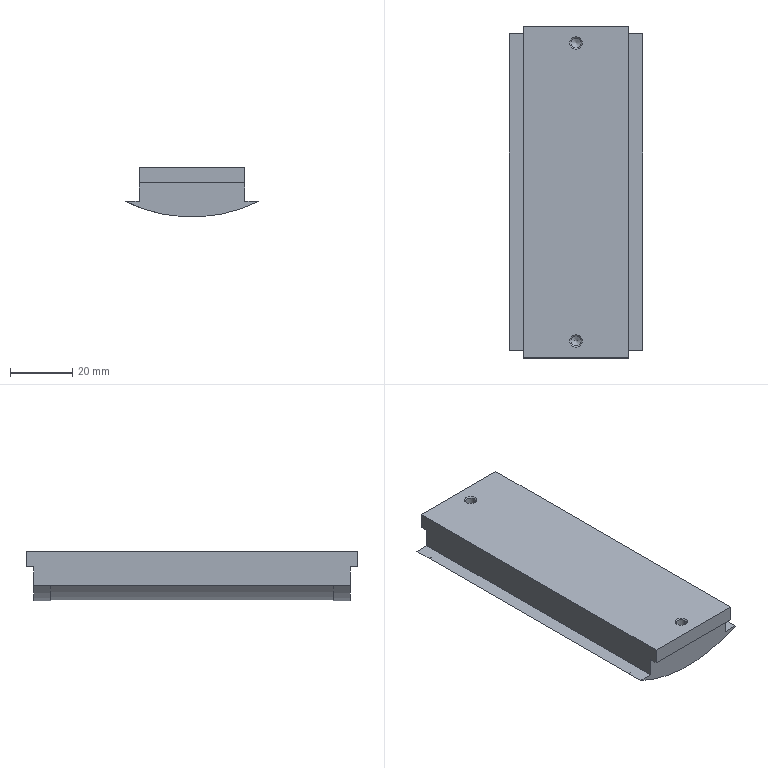Part | SolidWorks | features BaseBody 1, ICE 1 | 2 solids | 42 faces | box 43 x 107 x 16 mm | volume 22651 mm3 | cylinder 17 | plane 17 | cone 8 | commonest cylinder face diameters 3.242 x4 10 x4 56.416 x3 97.45 x3 19.866 x2 26 x1
STEP:
#1=CARTESIAN_POINT('',(-1.621,101.5,-0.379));
#2=VERTEX_POINT('',#1);
#3=CARTESIAN_POINT('',(1.621,101.5,-0.379));
#4=VERTEX_POINT('',#3);
#5=CARTESIAN_POINT('',(0.,101.5,-0.379));
#6=DIRECTION('',(0.,0.,1.));
#7=DIRECTION('',(1.,0.,0.));
#8=AXIS2_PLACEMENT_3D('',#5,#6,#7);
#9=CIRCLE('',#8,1.621);
#10=EDGE_CURVE('',#2,#4,#9,.T.);
#11=ORIENTED_EDGE('',*,*,#10,.F.);
#12=CARTESIAN_POINT('',(-2.,101.5,0.));
#13=VERTEX_POINT('',#12);
#14=CARTESIAN_POINT('',(-2.,101.5,0.));
#15=DIRECTION('',(-0.7071,0.,0.7071));
#16=VECTOR('',#15,1000.);
#17=LINE('',#14,#16);
#18=EDGE_CURVE('',#2,#13,#17,.T.);
#19=ORIENTED_EDGE('',*,*,#18,.T.);
#20=CARTESIAN_POINT('',(2.,101.5,0.));
#21=VERTEX_POINT('',#20);
#22=CARTESIAN_POINT('',(0.,101.5,0.));
#23=DIRECTION('',(0.,0.,1.));
#24=DIRECTION('',(1.,0.,0.));
#25=AXIS2_PLACEMENT_3D('',#22,#23,#24);
#26=CIRCLE('',#25,2.);
#27=EDGE_CURVE('',#13,#21,#26,.T.);
#28=ORIENTED_EDGE('',*,*,#27,.T.);
#29=CARTESIAN_POINT('',(2.,101.5,0.));
#30=DIRECTION('',(0.7071,0.,0.7071));
#31=VECTOR('',#30,1000.);
#32=LINE('',#29,#31);
#33=EDGE_CURVE('',#4,#21,#32,.T.);
#34=ORIENTED_EDGE('',*,*,#33,.F.);
#35=EDGE_LOOP('',(#11,#19,#28,#34));
#36=FACE_OUTER_BOUND('',#35,.T.);
#37=CARTESIAN_POINT('',(0.,101.5,0.));
#38=DIRECTION('',(0.,0.,1.));
#39=DIRECTION('',(1.,0.,0.));
#40=AXIS2_PLACEMENT_3D('',#37,#38,#39);
#41=CONICAL_SURFACE('',#40,2.,0.7854);
#42=ADVANCED_FACE('',(#36),#41,.F.);
#43=CARTESIAN_POINT('',(-1.621,5.5,-0.379));
#44=VERTEX_POINT('',#43);
#45=CARTESIAN_POINT('',(1.621,5.5,-0.379));
#46=VERTEX_POINT('',#45);
#47=CARTESIAN_POINT('',(0.,5.5,-0.379));
#48=DIRECTION('',(0.,0.,1.));
#49=DIRECTION('',(1.,0.,0.));
#50=AXIS2_PLACEMENT_3D('',#47,#48,#49);
#51=CIRCLE('',#50,1.621);
#52=EDGE_CURVE('',#44,#46,#51,.T.);
#53=ORIENTED_EDGE('',*,*,#52,.F.);
#54=CARTESIAN_POINT('',(-2.,5.5,0.));
#55=VERTEX_POINT('',#54);
#56=CARTESIAN_POINT('',(-2.,5.5,0.));
#57=DIRECTION('',(-0.7071,0.,0.7071));
#58=VECTOR('',#57,1000.);
#59=LINE('',#56,#58);
#60=EDGE_CURVE('',#44,#55,#59,.T.);
#61=ORIENTED_EDGE('',*,*,#60,.T.);
#62=CARTESIAN_POINT('',(2.,5.5,0.));
#63=VERTEX_POINT('',#62);
#64=CARTESIAN_POINT('',(0.,5.5,0.));
#65=DIRECTION('',(0.,0.,1.));
#66=DIRECTION('',(1.,0.,0.));
#67=AXIS2_PLACEMENT_3D('',#64,#65,#66);
#68=CIRCLE('',#67,2.);
#69=EDGE_CURVE('',#55,#63,#68,.T.);
#70=ORIENTED_EDGE('',*,*,#69,.T.);
#71=CARTESIAN_POINT('',(2.,5.5,0.));
#72=DIRECTION('',(0.7071,0.,0.7071));
#73=VECTOR('',#72,1000.);
#74=LINE('',#71,#73);
#75=EDGE_CURVE('',#46,#63,#74,.T.);
#76=ORIENTED_EDGE('',*,*,#75,.F.);
#77=EDGE_LOOP('',(#53,#61,#70,#76));
#78=FACE_OUTER_BOUND('',#77,.T.);
#79=CARTESIAN_POINT('',(0.,5.5,0.));
#80=DIRECTION('',(0.,0.,1.));
#81=DIRECTION('',(1.,0.,0.));
#82=AXIS2_PLACEMENT_3D('',#79,#80,#81);
#83=CONICAL_SURFACE('',#82,2.,0.7854);
#84=ADVANCED_FACE('',(#78),#83,.F.);
#85=CARTESIAN_POINT('',(-1.621,101.5,-6.219));
#86=VERTEX_POINT('',#85);
#87=CARTESIAN_POINT('',(1.621,101.5,-6.219));
#88=VERTEX_POINT('',#87);
#89=CARTESIAN_POINT('',(0.,101.5,-6.219));
#90=DIRECTION('',(0.,0.,1.));
#91=DIRECTION('',(1.,0.,0.));
#92=AXIS2_PLACEMENT_3D('',#89,#90,#91);
#93=CIRCLE('',#92,1.621);
#94=EDGE_CURVE('',#86,#88,#93,.T.);
#95=ORIENTED_EDGE('',*,*,#94,.F.);
#96=CARTESIAN_POINT('',(-1.621,101.5,-7.155));
#97=DIRECTION('',(0.,0.,1.));
#98=VECTOR('',#97,1000.);
#99=LINE('',#96,#98);
#100=EDGE_CURVE('',#86,#2,#99,.T.);
#101=ORIENTED_EDGE('',*,*,#100,.T.);
#102=ORIENTED_EDGE('',*,*,#10,.T.);
#103=CARTESIAN_POINT('',(1.621,101.5,-7.155));
#104=DIRECTION('',(0.,0.,1.));
#105=VECTOR('',#104,1000.);
#106=LINE('',#103,#105);
#107=EDGE_CURVE('',#88,#4,#106,.T.);
#108=ORIENTED_EDGE('',*,*,#107,.F.);
#109=EDGE_LOOP('',(#95,#101,#102,#108));
#110=FACE_OUTER_BOUND('',#109,.T.);
#111=CARTESIAN_POINT('',(0.,101.5,-7.155));
#112=DIRECTION('',(0.,0.,1.));
#113=DIRECTION('',(1.,0.,0.));
#114=AXIS2_PLACEMENT_3D('',#111,#112,#113);
#115=CYLINDRICAL_SURFACE('',#114,1.621);
#116=ADVANCED_FACE('',(#110),#115,.F.);
#117=CARTESIAN_POINT('',(-1.621,5.5,-6.219));
#118=VERTEX_POINT('',#117);
#119=CARTESIAN_POINT('',(1.621,5.5,-6.219));
#120=VERTEX_POINT('',#119);
#121=CARTESIAN_POINT('',(0.,5.5,-6.219));
#122=DIRECTION('',(0.,0.,1.));
#123=DIRECTION('',(1.,0.,0.));
#124=AXIS2_PLACEMENT_3D('',#121,#122,#123);
#125=CIRCLE('',#124,1.621);
#126=EDGE_CURVE('',#118,#120,#125,.T.);
#127=ORIENTED_EDGE('',*,*,#126,.F.);
#128=CARTESIAN_POINT('',(-1.621,5.5,-7.155));
#129=DIRECTION('',(0.,0.,1.));
#130=VECTOR('',#129,1000.);
#131=LINE('',#128,#130);
#132=EDGE_CURVE('',#118,#44,#131,.T.);
#133=ORIENTED_EDGE('',*,*,#132,.T.);
#134=ORIENTED_EDGE('',*,*,#52,.T.);
#135=CARTESIAN_POINT('',(1.621,5.5,-7.155));
#136=DIRECTION('',(0.,0.,1.));
#137=VECTOR('',#136,1000.);
#138=LINE('',#135,#137);
#139=EDGE_CURVE('',#120,#46,#138,.T.);
#140=ORIENTED_EDGE('',*,*,#139,.F.);
#141=EDGE_LOOP('',(#127,#133,#134,#140));
#142=FACE_OUTER_BOUND('',#141,.T.);
#143=CARTESIAN_POINT('',(0.,5.5,-7.155));
#144=DIRECTION('',(0.,0.,1.));
#145=DIRECTION('',(1.,0.,0.));
#146=AXIS2_PLACEMENT_3D('',#143,#144,#145);
#147=CYLINDRICAL_SURFACE('',#146,1.621);
#148=ADVANCED_FACE('',(#142),#147,.F.);
#149=CARTESIAN_POINT('',(0.,101.5,-7.155));
#150=VERTEX_POINT('',#149);
#151=CARTESIAN_POINT('',(1.621,101.5,-6.219));
#152=DIRECTION('',(0.866,0.,0.5));
#153=VECTOR('',#152,1000.);
#154=LINE('',#151,#153);
#155=EDGE_CURVE('',#150,#88,#154,.T.);
#156=ORIENTED_EDGE('',*,*,#155,.F.);
#157=CARTESIAN_POINT('',(-1.621,101.5,-6.219));
#158=DIRECTION('',(-0.866,0.,0.5));
#159=VECTOR('',#158,1000.);
#160=LINE('',#157,#159);
#161=EDGE_CURVE('',#150,#86,#160,.T.);
#162=ORIENTED_EDGE('',*,*,#161,.T.);
#163=ORIENTED_EDGE('',*,*,#94,.T.);
#164=EDGE_LOOP('',(#156,#162,#163));
#165=FACE_OUTER_BOUND('',#164,.T.);
#166=CARTESIAN_POINT('',(0.,101.5,-6.219));
#167=DIRECTION('',(0.,0.,1.));
#168=DIRECTION('',(1.,0.,0.));
#169=AXIS2_PLACEMENT_3D('',#166,#167,#168);
#170=CONICAL_SURFACE('',#169,1.621,1.047);
#171=ADVANCED_FACE('',(#165),#170,.F.);
#172=CARTESIAN_POINT('',(0.,5.5,-7.155));
#173=VERTEX_POINT('',#172);
#174=CARTESIAN_POINT('',(1.621,5.5,-6.219));
#175=DIRECTION('',(0.866,0.,0.5));
#176=VECTOR('',#175,1000.);
#177=LINE('',#174,#176);
#178=EDGE_CURVE('',#173,#120,#177,.T.);
#179=ORIENTED_EDGE('',*,*,#178,.F.);
#180=CARTESIAN_POINT('',(-1.621,5.5,-6.219));
#181=DIRECTION('',(-0.866,0.,0.5));
#182=VECTOR('',#181,1000.);
#183=LINE('',#180,#182);
#184=EDGE_CURVE('',#173,#118,#183,.T.);
#185=ORIENTED_EDGE('',*,*,#184,.T.);
#186=ORIENTED_EDGE('',*,*,#126,.T.);
#187=EDGE_LOOP('',(#179,#185,#186));
#188=FACE_OUTER_BOUND('',#187,.T.);
#189=CARTESIAN_POINT('',(0.,5.5,-6.219));
#190=DIRECTION('',(0.,0.,1.));
#191=DIRECTION('',(1.,0.,0.));
#192=AXIS2_PLACEMENT_3D('',#189,#190,#191);
#193=CONICAL_SURFACE('',#192,1.621,1.047);
#194=ADVANCED_FACE('',(#188),#193,.F.);
#195=CARTESIAN_POINT('',(0.,101.5,0.));
#196=DIRECTION('',(0.,0.,1.));
#197=DIRECTION('',(1.,0.,0.));
#198=AXIS2_PLACEMENT_3D('',#195,#196,#197);
#199=CIRCLE('',#198,2.);
#200=EDGE_CURVE('',#21,#13,#199,.T.);
#201=ORIENTED_EDGE('',*,*,#200,.F.);
#202=ORIENTED_EDGE('',*,*,#27,.F.);
#203=EDGE_LOOP('',(#201,#202));
#204=FACE_BOUND('',#203,.T.);
#205=CARTESIAN_POINT('',(17.,107.,0.));
#206=VERTEX_POINT('',#205);
#207=CARTESIAN_POINT('',(17.,0.,0.));
#208=VERTEX_POINT('',#207);
#209=CARTESIAN_POINT('',(17.,107.,0.));
#210=DIRECTION('',(0.,-1.,0.));
#211=VECTOR('',#210,1000.);
#212=LINE('',#209,#211);
#213=EDGE_CURVE('',#206,#208,#212,.T.);
#214=ORIENTED_EDGE('',*,*,#213,.F.);
#215=CARTESIAN_POINT('',(-17.,107.,0.));
#216=VERTEX_POINT('',#215);
#217=CARTESIAN_POINT('',(-17.,107.,0.));
#218=DIRECTION('',(1.,0.,0.));
#219=VECTOR('',#218,1000.);
#220=LINE('',#217,#219);
#221=EDGE_CURVE('',#216,#206,#220,.T.);
#222=ORIENTED_EDGE('',*,*,#221,.F.);
#223=CARTESIAN_POINT('',(-17.,0.,0.));
#224=VERTEX_POINT('',#223);
#225=CARTESIAN_POINT('',(-17.,107.,0.));
#226=DIRECTION('',(0.,1.,0.));
#227=VECTOR('',#226,1000.);
#228=LINE('',#225,#227);
#229=EDGE_CURVE('',#224,#216,#228,.T.);
#230=ORIENTED_EDGE('',*,*,#229,.F.);
#231=CARTESIAN_POINT('',(-17.,0.,0.));
#232=DIRECTION('',(-1.,0.,0.));
#233=VECTOR('',#232,1000.);
#234=LINE('',#231,#233);
#235=EDGE_CURVE('',#208,#224,#234,.T.);
#236=ORIENTED_EDGE('',*,*,#235,.F.);
#237=EDGE_LOOP('',(#214,#222,#230,#236));
#238=FACE_OUTER_BOUND('',#237,.T.);
#239=CARTESIAN_POINT('',(0.,5.5,0.));
#240=DIRECTION('',(0.,0.,1.));
#241=DIRECTION('',(1.,0.,0.));
#242=AXIS2_PLACEMENT_3D('',#239,#240,#241);
#243=CIRCLE('',#242,2.);
#244=EDGE_CURVE('',#63,#55,#243,.T.);
#245=ORIENTED_EDGE('',*,*,#244,.F.);
#246=ORIENTED_EDGE('',*,*,#69,.F.);
#247=EDGE_LOOP('',(#245,#246));
#248=FACE_BOUND('',#247,.T.);
#249=CARTESIAN_POINT('',(-17.,107.,0.));
#250=DIRECTION('',(0.,0.,-1.));
#251=DIRECTION('',(-1.,0.,0.));
#252=AXIS2_PLACEMENT_3D('',#249,#250,#251);
#253=PLANE('',#252);
#254=ADVANCED_FACE('',(#204,#238,#248),#253,.F.);
#255=ORIENTED_EDGE('',*,*,#18,.F.);
#256=CARTESIAN_POINT('',(0.,101.5,-0.379));
#257=DIRECTION('',(0.,0.,1.));
#258=DIRECTION('',(1.,0.,0.));
#259=AXIS2_PLACEMENT_3D('',#256,#257,#258);
#260=CIRCLE('',#259,1.621);
#261=EDGE_CURVE('',#4,#2,#260,.T.);
#262=ORIENTED_EDGE('',*,*,#261,.F.);
#263=ORIENTED_EDGE('',*,*,#33,.T.);
#264=ORIENTED_EDGE('',*,*,#200,.T.);
#265=EDGE_LOOP('',(#255,#262,#263,#264));
#266=FACE_OUTER_BOUND('',#265,.T.);
#267=CARTESIAN_POINT('',(0.,101.5,0.));
#268=DIRECTION('',(0.,0.,1.));
#269=DIRECTION('',(1.,0.,0.));
#270=AXIS2_PLACEMENT_3D('',#267,#268,#269);
#271=CONICAL_SURFACE('',#270,2.,0.7854);
#272=ADVANCED_FACE('',(#266),#271,.F.);
#273=CARTESIAN_POINT('',(17.,0.,-5.));
#274=VERTEX_POINT('',#273);
#275=CARTESIAN_POINT('',(17.,0.,32.725));
#276=DIRECTION('',(0.,0.,-1.));
#277=VECTOR('',#276,1000.);
#278=LINE('',#275,#277);
#279=EDGE_CURVE('',#208,#274,#278,.T.);
#280=ORIENTED_EDGE('',*,*,#279,.F.);
#281=ORIENTED_EDGE('',*,*,#235,.T.);
#282=CARTESIAN_POINT('',(-17.,0.,-5.));
#283=VERTEX_POINT('',#282);
#284=CARTESIAN_POINT('',(-17.,0.,32.725));
#285=DIRECTION('',(0.,0.,1.));
#286=VECTOR('',#285,1000.);
#287=LINE('',#284,#286);
#288=EDGE_CURVE('',#283,#224,#287,.T.);
#289=ORIENTED_EDGE('',*,*,#288,.F.);
#290=CARTESIAN_POINT('',(0.,0.,-5.));
#291=DIRECTION('',(-1.,0.,0.));
#292=VECTOR('',#291,1000.);
#293=LINE('',#290,#292);
#294=EDGE_CURVE('',#274,#283,#293,.T.);
#295=ORIENTED_EDGE('',*,*,#294,.F.);
#296=EDGE_LOOP('',(#280,#281,#289,#295));
#297=FACE_OUTER_BOUND('',#296,.T.);
#298=CARTESIAN_POINT('',(0.,0.,32.725));
#299=DIRECTION('',(0.,1.,0.));
#300=DIRECTION('',(0.,0.,1.));
#301=AXIS2_PLACEMENT_3D('',#298,#299,#300);
#302=PLANE('',#301);
#303=ADVANCED_FACE('',(#297),#302,.F.);
#304=CARTESIAN_POINT('',(17.,104.5,-11.));
#305=VERTEX_POINT('',#304);
#306=CARTESIAN_POINT('',(17.,2.5,-11.));
#307=VERTEX_POINT('',#306);
#308=CARTESIAN_POINT('',(17.,107.,-11.));
#309=DIRECTION('',(0.,-1.,0.));
#310=VECTOR('',#309,1000.);
#311=LINE('',#308,#310);
#312=EDGE_CURVE('',#305,#307,#311,.T.);
#313=ORIENTED_EDGE('',*,*,#312,.F.);
#314=CARTESIAN_POINT('',(17.,104.5,-5.));
#315=VERTEX_POINT('',#314);
#316=CARTESIAN_POINT('',(17.,104.5,0.));
#317=DIRECTION('',(0.,0.,-1.));
#318=VECTOR('',#317,1000.);
#319=LINE('',#316,#318);
#320=EDGE_CURVE('',#315,#305,#319,.T.);
#321=ORIENTED_EDGE('',*,*,#320,.F.);
#322=CARTESIAN_POINT('',(17.,107.,-5.));
#323=VERTEX_POINT('',#322);
#324=CARTESIAN_POINT('',(17.,107.,-5.));
#325=DIRECTION('',(0.,-1.,0.));
#326=VECTOR('',#325,1000.);
#327=LINE('',#324,#326);
#328=EDGE_CURVE('',#323,#315,#327,.T.);
#329=ORIENTED_EDGE('',*,*,#328,.F.);
#330=CARTESIAN_POINT('',(17.,107.,0.));
#331=DIRECTION('',(0.,0.,-1.));
#332=VECTOR('',#331,1000.);
#333=LINE('',#330,#332);
#334=EDGE_CURVE('',#206,#323,#333,.T.);
#335=ORIENTED_EDGE('',*,*,#334,.F.);
#336=ORIENTED_EDGE('',*,*,#213,.T.);
#337=ORIENTED_EDGE('',*,*,#279,.T.);
#338=CARTESIAN_POINT('',(17.,2.5,-5.));
#339=VERTEX_POINT('',#338);
#340=CARTESIAN_POINT('',(17.,107.,-5.));
#341=DIRECTION('',(0.,-1.,0.));
#342=VECTOR('',#341,1000.);
#343=LINE('',#340,#342);
#344=EDGE_CURVE('',#339,#274,#343,.T.);
#345=ORIENTED_EDGE('',*,*,#344,.F.);
#346=CARTESIAN_POINT('',(17.,2.5,0.));
#347=DIRECTION('',(0.,0.,1.));
#348=VECTOR('',#347,1000.);
#349=LINE('',#346,#348);
#350=EDGE_CURVE('',#307,#339,#349,.T.);
#351=ORIENTED_EDGE('',*,*,#350,.F.);
#352=EDGE_LOOP('',(#313,#321,#329,#335,#336,#337,#345,#351));
#353=FACE_OUTER_BOUND('',#352,.T.);
#354=CARTESIAN_POINT('',(17.,107.,0.));
#355=DIRECTION('',(-1.,0.,0.));
#356=DIRECTION('',(0.,0.,1.));
#357=AXIS2_PLACEMENT_3D('',#354,#355,#356);
#358=PLANE('',#357);
#359=ADVANCED_FACE('',(#353),#358,.F.);
#360=CARTESIAN_POINT('',(-17.,107.,-5.));
#361=VERTEX_POINT('',#360);
#362=CARTESIAN_POINT('',(-17.,107.,32.725));
#363=DIRECTION('',(0.,0.,1.));
#364=VECTOR('',#363,1000.);
#365=LINE('',#362,#364);
#366=EDGE_CURVE('',#361,#216,#365,.T.);
#367=ORIENTED_EDGE('',*,*,#366,.T.);
#368=ORIENTED_EDGE('',*,*,#221,.T.);
#369=ORIENTED_EDGE('',*,*,#334,.T.);
#370=CARTESIAN_POINT('',(0.,107.,-5.));
#371=DIRECTION('',(-1.,0.,0.));
#372=VECTOR('',#371,1000.);
#373=LINE('',#370,#372);
#374=EDGE_CURVE('',#323,#361,#373,.T.);
#375=ORIENTED_EDGE('',*,*,#374,.T.);
#376=EDGE_LOOP('',(#367,#368,#369,#375));
#377=FACE_OUTER_BOUND('',#376,.T.);
#378=CARTESIAN_POINT('',(0.,107.,32.725));
#379=DIRECTION('',(0.,1.,0.));
#380=DIRECTION('',(0.,0.,1.));
#381=AXIS2_PLACEMENT_3D('',#378,#379,#380);
#382=PLANE('',#381);
#383=ADVANCED_FACE('',(#377),#382,.T.);
#384=CARTESIAN_POINT('',(-17.,2.5,-5.));
#385=VERTEX_POINT('',#384);
#386=CARTESIAN_POINT('',(-17.,107.,-5.));
#387=DIRECTION('',(0.,1.,0.));
#388=VECTOR('',#387,1000.);
#389=LINE('',#386,#388);
#390=EDGE_CURVE('',#283,#385,#389,.T.);
#391=ORIENTED_EDGE('',*,*,#390,.F.);
#392=ORIENTED_EDGE('',*,*,#288,.T.);
#393=ORIENTED_EDGE('',*,*,#229,.T.);
#394=ORIENTED_EDGE('',*,*,#366,.F.);
#395=CARTESIAN_POINT('',(-17.,104.5,-5.));
#396=VERTEX_POINT('',#395);
#397=CARTESIAN_POINT('',(-17.,107.,-5.));
#398=DIRECTION('',(0.,1.,0.));
#399=VECTOR('',#398,1000.);
#400=LINE('',#397,#399);
#401=EDGE_CURVE('',#396,#361,#400,.T.);
#402=ORIENTED_EDGE('',*,*,#401,.F.);
#403=CARTESIAN_POINT('',(-17.,104.5,-11.));
#404=VERTEX_POINT('',#403);
#405=CARTESIAN_POINT('',(-17.,104.5,-11.));
#406=DIRECTION('',(0.,0.,1.));
#407=VECTOR('',#406,1000.);
#408=LINE('',#405,#407);
#409=EDGE_CURVE('',#404,#396,#408,.T.);
#410=ORIENTED_EDGE('',*,*,#409,.F.);
#411=CARTESIAN_POINT('',(-17.,2.5,-11.));
#412=VERTEX_POINT('',#411);
#413=CARTESIAN_POINT('',(-17.,107.,-11.));
#414=DIRECTION('',(0.,1.,0.));
#415=VECTOR('',#414,1000.);
#416=LINE('',#413,#415);
#417=EDGE_CURVE('',#412,#404,#416,.T.);
#418=ORIENTED_EDGE('',*,*,#417,.F.);
#419=CARTESIAN_POINT('',(-17.,2.5,-11.));
#420=DIRECTION('',(0.,0.,-1.));
#421=VECTOR('',#420,1000.);
#422=LINE('',#419,#421);
#423=EDGE_CURVE('',#385,#412,#422,.T.);
#424=ORIENTED_EDGE('',*,*,#423,.F.);
#425=EDGE_LOOP('',(#391,#392,#393,#394,#402,#410,#418,#424));
#426=FACE_OUTER_BOUND('',#425,.T.);
#427=CARTESIAN_POINT('',(-17.,107.,-11.));
#428=DIRECTION('',(1.,0.,0.));
#429=DIRECTION('',(0.,0.,-1.));
#430=AXIS2_PLACEMENT_3D('',#427,#428,#429);
#431=PLANE('',#430);
#432=ADVANCED_FACE('',(#426),#431,.F.);
#433=ORIENTED_EDGE('',*,*,#60,.F.);
#434=CARTESIAN_POINT('',(0.,5.5,-0.379));
#435=DIRECTION('',(0.,0.,1.));
#436=DIRECTION('',(1.,0.,0.));
#437=AXIS2_PLACEMENT_3D('',#434,#435,#436);
#438=CIRCLE('',#437,1.621);
#439=EDGE_CURVE('',#46,#44,#438,.T.);
#440=ORIENTED_EDGE('',*,*,#439,.F.);
#441=ORIENTED_EDGE('',*,*,#75,.T.);
#442=ORIENTED_EDGE('',*,*,#244,.T.);
#443=EDGE_LOOP('',(#433,#440,#441,#442));
#444=FACE_OUTER_BOUND('',#443,.T.);
#445=CARTESIAN_POINT('',(0.,5.5,0.));
#446=DIRECTION('',(0.,0.,1.));
#447=DIRECTION('',(1.,0.,0.));
#448=AXIS2_PLACEMENT_3D('',#445,#446,#447);
#449=CONICAL_SURFACE('',#448,2.,0.7854);
#450=ADVANCED_FACE('',(#444),#449,.F.);
#451=ORIENTED_EDGE('',*,*,#100,.F.);
#452=CARTESIAN_POINT('',(0.,101.5,-6.219));
#453=DIRECTION('',(0.,0.,1.));
#454=DIRECTION('',(1.,0.,0.));
#455=AXIS2_PLACEMENT_3D('',#452,#453,#454);
#456=CIRCLE('',#455,1.621);
#457=EDGE_CURVE('',#88,#86,#456,.T.);
#458=ORIENTED_EDGE('',*,*,#457,.F.);
#459=ORIENTED_EDGE('',*,*,#107,.T.);
#460=ORIENTED_EDGE('',*,*,#261,.T.);
#461=EDGE_LOOP('',(#451,#458,#459,#460));
#462=FACE_OUTER_BOUND('',#461,.T.);
#463=CARTESIAN_POINT('',(0.,101.5,-7.155));
#464=DIRECTION('',(0.,0.,1.));
#465=DIRECTION('',(1.,0.,0.));
#466=AXIS2_PLACEMENT_3D('',#463,#464,#465);
#467=CYLINDRICAL_SURFACE('',#466,1.621);
#468=ADVANCED_FACE('',(#462),#467,.F.);
#469=ORIENTED_EDGE('',*,*,#344,.T.);
#470=ORIENTED_EDGE('',*,*,#294,.T.);
#471=ORIENTED_EDGE('',*,*,#390,.T.);
#472=CARTESIAN_POINT('',(22.,2.5,-5.));
#473=DIRECTION('',(1.,0.,0.));
#474=VECTOR('',#473,1000.);
#475=LINE('',#472,#474);
#476=EDGE_CURVE('',#385,#339,#475,.T.);
#477=ORIENTED_EDGE('',*,*,#476,.T.);
#478=EDGE_LOOP('',(#469,#470,#471,#477));
#479=FACE_OUTER_BOUND('',#478,.T.);
#480=CARTESIAN_POINT('',(22.,2.5,-5.));
#481=DIRECTION('',(0.,0.,-1.));
#482=DIRECTION('',(0.,1.,0.));
#483=AXIS2_PLACEMENT_3D('',#480,#481,#482);
#484=PLANE('',#483);
#485=ADVANCED_FACE('',(#479),#484,.T.);
#486=ORIENTED_EDGE('',*,*,#350,.T.);
#487=ORIENTED_EDGE('',*,*,#476,.F.);
#488=ORIENTED_EDGE('',*,*,#423,.T.);
#489=CARTESIAN_POINT('',(-21.5,2.5,-11.));
#490=VERTEX_POINT('',#489);
#491=CARTESIAN_POINT('',(22.,2.5,-11.));
#492=DIRECTION('',(-1.,0.,0.));
#493=VECTOR('',#492,1000.);
#494=LINE('',#491,#493);
#495=EDGE_CURVE('',#412,#490,#494,.T.);
#496=ORIENTED_EDGE('',*,*,#495,.T.);
#497=CARTESIAN_POINT('',(21.5,2.5,-11.));
#498=VERTEX_POINT('',#497);
#499=CARTESIAN_POINT('',(0.,2.5,32.725));
#500=DIRECTION('',(0.,-1.,0.));
#501=DIRECTION('',(0.,0.,1.));
#502=AXIS2_PLACEMENT_3D('',#499,#500,#501);
#503=CIRCLE('',#502,48.725);
#504=EDGE_CURVE('',#490,#498,#503,.T.);
#505=ORIENTED_EDGE('',*,*,#504,.T.);
#506=CARTESIAN_POINT('',(22.,2.5,-11.));
#507=DIRECTION('',(-1.,0.,0.));
#508=VECTOR('',#507,1000.);
#509=LINE('',#506,#508);
#510=EDGE_CURVE('',#498,#307,#509,.T.);
#511=ORIENTED_EDGE('',*,*,#510,.T.);
#512=EDGE_LOOP('',(#486,#487,#488,#496,#505,#511));
#513=FACE_OUTER_BOUND('',#512,.T.);
#514=CARTESIAN_POINT('',(22.,2.5,-17.));
#515=DIRECTION('',(0.,-1.,0.));
#516=DIRECTION('',(0.,0.,-1.));
#517=AXIS2_PLACEMENT_3D('',#514,#515,#516);
#518=PLANE('',#517);
#519=ADVANCED_FACE('',(#513),#518,.T.);
#520=CARTESIAN_POINT('',(21.5,8.,-11.));
#521=VERTEX_POINT('',#520);
#522=CARTESIAN_POINT('',(21.5,107.,-11.));
#523=DIRECTION('',(0.,-1.,0.));
#524=VECTOR('',#523,1000.);
#525=LINE('',#522,#524);
#526=EDGE_CURVE('',#521,#498,#525,.T.);
#527=ORIENTED_EDGE('',*,*,#526,.F.);
#528=CARTESIAN_POINT('',(21.5,99.,-11.));
#529=VERTEX_POINT('',#528);
#530=CARTESIAN_POINT('',(21.5,107.,-11.));
#531=DIRECTION('',(0.,-1.,0.));
#532=VECTOR('',#531,1000.);
#533=LINE('',#530,#532);
#534=EDGE_CURVE('',#529,#521,#533,.T.);
#535=ORIENTED_EDGE('',*,*,#534,.F.);
#536=CARTESIAN_POINT('',(21.5,104.5,-11.));
#537=VERTEX_POINT('',#536);
#538=CARTESIAN_POINT('',(21.5,107.,-11.));
#539=DIRECTION('',(0.,-1.,0.));
#540=VECTOR('',#539,1000.);
#541=LINE('',#538,#540);
#542=EDGE_CURVE('',#537,#529,#541,.T.);
#543=ORIENTED_EDGE('',*,*,#542,.F.);
#544=CARTESIAN_POINT('',(17.,104.5,-11.));
#545=DIRECTION('',(1.,0.,0.));
#546=VECTOR('',#545,1000.);
#547=LINE('',#544,#546);
#548=EDGE_CURVE('',#305,#537,#547,.T.);
#549=ORIENTED_EDGE('',*,*,#548,.F.);
#550=ORIENTED_EDGE('',*,*,#312,.T.);
#551=ORIENTED_EDGE('',*,*,#510,.F.);
#552=EDGE_LOOP('',(#527,#535,#543,#549,#550,#551));
#553=FACE_OUTER_BOUND('',#552,.T.);
#554=CARTESIAN_POINT('',(17.,107.,-11.));
#555=DIRECTION('',(0.,0.,-1.));
#556=DIRECTION('',(-1.,0.,0.));
#557=AXIS2_PLACEMENT_3D('',#554,#555,#556);
#558=PLANE('',#557);
#559=ADVANCED_FACE('',(#553),#558,.F.);
#560=CARTESIAN_POINT('',(-21.5,104.5,-11.));
#561=VERTEX_POINT('',#560);
#562=CARTESIAN_POINT('',(0.,104.5,32.725));
#563=DIRECTION('',(0.,1.,0.));
#564=DIRECTION('',(0.,0.,1.));
#565=AXIS2_PLACEMENT_3D('',#562,#563,#564);
#566=CIRCLE('',#565,48.725);
#567=EDGE_CURVE('',#537,#561,#566,.T.);
#568=ORIENTED_EDGE('',*,*,#567,.T.);
#569=CARTESIAN_POINT('',(22.,104.5,-11.));
#570=DIRECTION('',(1.,0.,0.));
#571=VECTOR('',#570,1000.);
#572=LINE('',#569,#571);
#573=EDGE_CURVE('',#561,#404,#572,.T.);
#574=ORIENTED_EDGE('',*,*,#573,.T.);
#575=ORIENTED_EDGE('',*,*,#409,.T.);
#576=CARTESIAN_POINT('',(22.,104.5,-5.));
#577=DIRECTION('',(1.,0.,0.));
#578=VECTOR('',#577,1000.);
#579=LINE('',#576,#578);
#580=EDGE_CURVE('',#396,#315,#579,.T.);
#581=ORIENTED_EDGE('',*,*,#580,.T.);
#582=ORIENTED_EDGE('',*,*,#320,.T.);
#583=ORIENTED_EDGE('',*,*,#548,.T.);
#584=EDGE_LOOP('',(#568,#574,#575,#581,#582,#583));
#585=FACE_OUTER_BOUND('',#584,.T.);
#586=CARTESIAN_POINT('',(22.,104.5,-5.));
#587=DIRECTION('',(0.,1.,0.));
#588=DIRECTION('',(0.,0.,1.));
#589=AXIS2_PLACEMENT_3D('',#586,#587,#588);
#590=PLANE('',#589);
#591=ADVANCED_FACE('',(#585),#590,.T.);
#592=ORIENTED_EDGE('',*,*,#328,.T.);
#593=ORIENTED_EDGE('',*,*,#580,.F.);
#594=ORIENTED_EDGE('',*,*,#401,.T.);
#595=ORIENTED_EDGE('',*,*,#374,.F.);
#596=EDGE_LOOP('',(#592,#593,#594,#595));
#597=FACE_OUTER_BOUND('',#596,.T.);
#598=CARTESIAN_POINT('',(22.,107.,-5.));
#599=DIRECTION('',(0.,0.,-1.));
#600=DIRECTION('',(-1.,0.,0.));
#601=AXIS2_PLACEMENT_3D('',#598,#599,#600);
#602=PLANE('',#601);
#603=ADVANCED_FACE('',(#597),#602,.T.);
#604=ORIENTED_EDGE('',*,*,#417,.T.);
#605=ORIENTED_EDGE('',*,*,#573,.F.);
#606=CARTESIAN_POINT('',(-21.5,99.,-11.));
#607=VERTEX_POINT('',#606);
#608=CARTESIAN_POINT('',(-21.5,107.,-11.));
#609=DIRECTION('',(0.,1.,0.));
#610=VECTOR('',#609,1000.);
#611=LINE('',#608,#610);
#612=EDGE_CURVE('',#607,#561,#611,.T.);
#613=ORIENTED_EDGE('',*,*,#612,.F.);
#614=CARTESIAN_POINT('',(-21.5,8.,-11.));
#615=VERTEX_POINT('',#614);
#616=CARTESIAN_POINT('',(-21.5,107.,-11.));
#617=DIRECTION('',(0.,1.,0.));
#618=VECTOR('',#617,1000.);
#619=LINE('',#616,#618);
#620=EDGE_CURVE('',#615,#607,#619,.T.);
#621=ORIENTED_EDGE('',*,*,#620,.F.);
#622=CARTESIAN_POINT('',(-21.5,107.,-11.));
#623=DIRECTION('',(0.,1.,0.));
#624=VECTOR('',#623,1000.);
#625=LINE('',#622,#624);
#626=EDGE_CURVE('',#490,#615,#625,.T.);
#627=ORIENTED_EDGE('',*,*,#626,.F.);
#628=ORIENTED_EDGE('',*,*,#495,.F.);
#629=EDGE_LOOP('',(#604,#605,#613,#621,#627,#628));
#630=FACE_OUTER_BOUND('',#629,.T.);
#631=CARTESIAN_POINT('',(-21.5,107.,-11.));
#632=DIRECTION('',(0.,0.,-1.));
#633=DIRECTION('',(-1.,0.,0.));
#634=AXIS2_PLACEMENT_3D('',#631,#632,#633);
#635=PLANE('',#634);
#636=ADVANCED_FACE('',(#630),#635,.F.);
#637=ORIENTED_EDGE('',*,*,#132,.F.);
#638=CARTESIAN_POINT('',(0.,5.5,-6.219));
#639=DIRECTION('',(0.,0.,1.));
#640=DIRECTION('',(1.,0.,0.));
#641=AXIS2_PLACEMENT_3D('',#638,#639,#640);
#642=CIRCLE('',#641,1.621);
#643=EDGE_CURVE('',#120,#118,#642,.T.);
#644=ORIENTED_EDGE('',*,*,#643,.F.);
#645=ORIENTED_EDGE('',*,*,#139,.T.);
#646=ORIENTED_EDGE('',*,*,#439,.T.);
#647=EDGE_LOOP('',(#637,#644,#645,#646));
#648=FACE_OUTER_BOUND('',#647,.T.);
#649=CARTESIAN_POINT('',(0.,5.5,-7.155));
#650=DIRECTION('',(0.,0.,1.));
#651=DIRECTION('',(1.,0.,0.));
#652=AXIS2_PLACEMENT_3D('',#649,#650,#651);
#653=CYLINDRICAL_SURFACE('',#652,1.621);
#654=ADVANCED_FACE('',(#648),#653,.F.);
#655=ORIENTED_EDGE('',*,*,#161,.F.);
#656=ORIENTED_EDGE('',*,*,#155,.T.);
#657=ORIENTED_EDGE('',*,*,#457,.T.);
#658=EDGE_LOOP('',(#655,#656,#657));
#659=FACE_OUTER_BOUND('',#658,.T.);
#660=CARTESIAN_POINT('',(0.,101.5,-6.219));
#661=DIRECTION('',(0.,0.,1.));
#662=DIRECTION('',(1.,0.,0.));
#663=AXIS2_PLACEMENT_3D('',#660,#661,#662);
#664=CONICAL_SURFACE('',#663,1.621,1.047);
#665=ADVANCED_FACE('',(#659),#664,.F.);
#666=CARTESIAN_POINT('',(0.,8.,32.725));
#667=DIRECTION('',(0.,-1.,0.));
#668=DIRECTION('',(0.,0.,1.));
#669=AXIS2_PLACEMENT_3D('',#666,#667,#668);
#670=CIRCLE('',#669,48.725);
#671=EDGE_CURVE('',#615,#521,#670,.T.);
#672=ORIENTED_EDGE('',*,*,#671,.T.);
#673=ORIENTED_EDGE('',*,*,#526,.T.);
#674=ORIENTED_EDGE('',*,*,#504,.F.);
#675=ORIENTED_EDGE('',*,*,#626,.T.);
#676=EDGE_LOOP('',(#672,#673,#674,#675));
#677=FACE_OUTER_BOUND('',#676,.T.);
#678=CARTESIAN_POINT('',(0.,107.,32.725));
#679=DIRECTION('',(0.,1.,0.));
#680=DIRECTION('',(0.,0.,1.));
#681=AXIS2_PLACEMENT_3D('',#678,#679,#680);
#682=CYLINDRICAL_SURFACE('',#681,48.725);
#683=ADVANCED_FACE('',(#677),#682,.T.);
#684=CARTESIAN_POINT('',(18.673,99.,-11.618));
#685=VERTEX_POINT('',#684);
#686=CARTESIAN_POINT('',(14.07,99.,16.212));
#687=DIRECTION('',(0.,-1.,0.));
#688=DIRECTION('',(0.,0.,1.));
#689=AXIS2_PLACEMENT_3D('',#686,#687,#688);
#690=CIRCLE('',#689,28.208);
#691=EDGE_CURVE('',#685,#529,#690,.T.);
#692=ORIENTED_EDGE('',*,*,#691,.T.);
#693=ORIENTED_EDGE('',*,*,#534,.T.);
#694=CARTESIAN_POINT('',(18.673,8.,-11.618));
#695=VERTEX_POINT('',#694);
#696=CARTESIAN_POINT('',(14.07,8.,16.212));
#697=DIRECTION('',(0.,1.,0.));
#698=DIRECTION('',(0.,0.,1.));
#699=AXIS2_PLACEMENT_3D('',#696,#697,#698);
#700=CIRCLE('',#699,28.208);
#701=EDGE_CURVE('',#521,#695,#700,.T.);
#702=ORIENTED_EDGE('',*,*,#701,.T.);
#703=CARTESIAN_POINT('',(18.673,99.,-11.618));
#704=DIRECTION('',(0.,1.,0.));
#705=VECTOR('',#704,1000.);
#706=LINE('',#703,#705);
#707=EDGE_CURVE('',#695,#685,#706,.T.);
#708=ORIENTED_EDGE('',*,*,#707,.T.);
#709=EDGE_LOOP('',(#692,#693,#702,#708));
#710=FACE_OUTER_BOUND('',#709,.T.);
#711=CARTESIAN_POINT('',(14.07,99.,16.212));
#712=DIRECTION('',(0.,1.,0.));
#713=DIRECTION('',(0.,0.,1.));
#714=AXIS2_PLACEMENT_3D('',#711,#712,#713);
#715=CYLINDRICAL_SURFACE('',#714,28.208);
#716=ADVANCED_FACE('',(#710),#715,.T.);
#717=CARTESIAN_POINT('',(0.,99.,32.725));
#718=DIRECTION('',(0.,1.,0.));
#719=DIRECTION('',(0.,0.,1.));
#720=AXIS2_PLACEMENT_3D('',#717,#718,#719);
#721=CIRCLE('',#720,48.725);
#722=EDGE_CURVE('',#529,#607,#721,.T.);
#723=ORIENTED_EDGE('',*,*,#722,.T.);
#724=ORIENTED_EDGE('',*,*,#612,.T.);
#725=ORIENTED_EDGE('',*,*,#567,.F.);
#726=ORIENTED_EDGE('',*,*,#542,.T.);
#727=EDGE_LOOP('',(#723,#724,#725,#726));
#728=FACE_OUTER_BOUND('',#727,.T.);
#729=CARTESIAN_POINT('',(0.,107.,32.725));
#730=DIRECTION('',(0.,1.,0.));
#731=DIRECTION('',(0.,0.,1.));
#732=AXIS2_PLACEMENT_3D('',#729,#730,#731);
#733=CYLINDRICAL_SURFACE('',#732,48.725);
#734=ADVANCED_FACE('',(#728),#733,.T.);
#735=CARTESIAN_POINT('',(-18.672,99.,-11.618));
#736=VERTEX_POINT('',#735);
#737=CARTESIAN_POINT('',(-14.072,99.,16.212));
#738=DIRECTION('',(0.,-1.,0.));
#739=DIRECTION('',(0.,0.,1.));
#740=AXIS2_PLACEMENT_3D('',#737,#738,#739);
#741=CIRCLE('',#740,28.208);
#742=EDGE_CURVE('',#607,#736,#741,.T.);
#743=ORIENTED_EDGE('',*,*,#742,.T.);
#744=CARTESIAN_POINT('',(-18.672,8.,-11.618));
#745=VERTEX_POINT('',#744);
#746=CARTESIAN_POINT('',(-18.672,99.,-11.618));
#747=DIRECTION('',(0.,-1.,0.));
#748=VECTOR('',#747,1000.);
#749=LINE('',#746,#748);
#750=EDGE_CURVE('',#736,#745,#749,.T.);
#751=ORIENTED_EDGE('',*,*,#750,.T.);
#752=CARTESIAN_POINT('',(-14.072,8.,16.212));
#753=DIRECTION('',(0.,1.,0.));
#754=DIRECTION('',(0.,0.,1.));
#755=AXIS2_PLACEMENT_3D('',#752,#753,#754);
#756=CIRCLE('',#755,28.208);
#757=EDGE_CURVE('',#745,#615,#756,.T.);
#758=ORIENTED_EDGE('',*,*,#757,.T.);
#759=ORIENTED_EDGE('',*,*,#620,.T.);
#760=EDGE_LOOP('',(#743,#751,#758,#759));
#761=FACE_OUTER_BOUND('',#760,.T.);
#762=CARTESIAN_POINT('',(-14.072,99.,16.212));
#763=DIRECTION('',(0.,1.,0.));
#764=DIRECTION('',(0.,0.,1.));
#765=AXIS2_PLACEMENT_3D('',#762,#763,#764);
#766=CYLINDRICAL_SURFACE('',#765,28.208);
#767=ADVANCED_FACE('',(#761),#766,.T.);
#768=ORIENTED_EDGE('',*,*,#184,.F.);
#769=ORIENTED_EDGE('',*,*,#178,.T.);
#770=ORIENTED_EDGE('',*,*,#643,.T.);
#771=EDGE_LOOP('',(#768,#769,#770));
#772=FACE_OUTER_BOUND('',#771,.T.);
#773=CARTESIAN_POINT('',(0.,5.5,-6.219));
#774=DIRECTION('',(0.,0.,1.));
#775=DIRECTION('',(1.,0.,0.));
#776=AXIS2_PLACEMENT_3D('',#773,#774,#775);
#777=CONICAL_SURFACE('',#776,1.621,1.047);
#778=ADVANCED_FACE('',(#772),#777,.F.);
#779=CARTESIAN_POINT('',(13.093,8.,-8.202));
#780=VERTEX_POINT('',#779);
#781=CARTESIAN_POINT('',(17.857,8.,-6.685));
#782=DIRECTION('',(0.,-1.,0.));
#783=DIRECTION('',(0.,0.,1.));
#784=AXIS2_PLACEMENT_3D('',#781,#782,#783);
#785=CIRCLE('',#784,5.);
#786=EDGE_CURVE('',#780,#695,#785,.T.);
#787=ORIENTED_EDGE('',*,*,#786,.T.);
#788=ORIENTED_EDGE('',*,*,#701,.F.);
#789=ORIENTED_EDGE('',*,*,#671,.F.);
#790=ORIENTED_EDGE('',*,*,#757,.F.);
#791=CARTESIAN_POINT('',(-13.092,8.,-8.202));
#792=VERTEX_POINT('',#791);
#793=CARTESIAN_POINT('',(-17.856,8.,-6.685));
#794=DIRECTION('',(0.,-1.,0.));
#795=DIRECTION('',(0.,0.,1.));
#796=AXIS2_PLACEMENT_3D('',#793,#794,#795);
#797=CIRCLE('',#796,5.);
#798=EDGE_CURVE('',#745,#792,#797,.T.);
#799=ORIENTED_EDGE('',*,*,#798,.T.);
#800=CARTESIAN_POINT('',(-5.691,8.,-1.5));
#801=VERTEX_POINT('',#800);
#802=CARTESIAN_POINT('',(-3.627,8.,-11.216));
#803=DIRECTION('',(0.,1.,0.));
#804=DIRECTION('',(0.,0.,1.));
#805=AXIS2_PLACEMENT_3D('',#802,#803,#804);
#806=CIRCLE('',#805,9.933);
#807=EDGE_CURVE('',#792,#801,#806,.T.);
#808=ORIENTED_EDGE('',*,*,#807,.T.);
#809=CARTESIAN_POINT('',(5.692,8.,-1.5));
#810=VERTEX_POINT('',#809);
#811=CARTESIAN_POINT('',(-14.072,8.,-1.5));
#812=DIRECTION('',(1.,0.,0.));
#813=VECTOR('',#812,1000.);
#814=LINE('',#811,#813);
#815=EDGE_CURVE('',#801,#810,#814,.T.);
#816=ORIENTED_EDGE('',*,*,#815,.T.);
#817=CARTESIAN_POINT('',(3.628,8.,-11.216));
#818=DIRECTION('',(0.,1.,0.));
#819=DIRECTION('',(0.,0.,1.));
#820=AXIS2_PLACEMENT_3D('',#817,#818,#819);
#821=CIRCLE('',#820,9.933);
#822=EDGE_CURVE('',#810,#780,#821,.T.);
#823=ORIENTED_EDGE('',*,*,#822,.T.);
#824=EDGE_LOOP('',(#787,#788,#789,#790,#799,#808,#816,#823));
#825=FACE_OUTER_BOUND('',#824,.T.);
#826=CARTESIAN_POINT('',(-14.072,8.,16.212));
#827=DIRECTION('',(0.,1.,0.));
#828=DIRECTION('',(0.,0.,1.));
#829=AXIS2_PLACEMENT_3D('',#826,#827,#828);
#830=PLANE('',#829);
#831=ADVANCED_FACE('',(#825),#830,.T.);
#832=CARTESIAN_POINT('',(13.093,99.,-8.202));
#833=VERTEX_POINT('',#832);
#834=CARTESIAN_POINT('',(17.857,99.,-6.685));
#835=DIRECTION('',(0.,-1.,0.));
#836=DIRECTION('',(0.,0.,1.));
#837=AXIS2_PLACEMENT_3D('',#834,#835,#836);
#838=CIRCLE('',#837,5.);
#839=EDGE_CURVE('',#833,#685,#838,.T.);
#840=ORIENTED_EDGE('',*,*,#839,.F.);
#841=CARTESIAN_POINT('',(5.692,99.,-1.5));
#842=VERTEX_POINT('',#841);
#843=CARTESIAN_POINT('',(3.628,99.,-11.216));
#844=DIRECTION('',(0.,1.,0.));
#845=DIRECTION('',(0.,0.,1.));
#846=AXIS2_PLACEMENT_3D('',#843,#844,#845);
#847=CIRCLE('',#846,9.933);
#848=EDGE_CURVE('',#842,#833,#847,.T.);
#849=ORIENTED_EDGE('',*,*,#848,.F.);
#850=CARTESIAN_POINT('',(-5.691,99.,-1.5));
#851=VERTEX_POINT('',#850);
#852=CARTESIAN_POINT('',(-14.072,99.,-1.5));
#853=DIRECTION('',(1.,0.,0.));
#854=VECTOR('',#853,1000.);
#855=LINE('',#852,#854);
#856=EDGE_CURVE('',#851,#842,#855,.T.);
#857=ORIENTED_EDGE('',*,*,#856,.F.);
#858=CARTESIAN_POINT('',(-13.092,99.,-8.202));
#859=VERTEX_POINT('',#858);
#860=CARTESIAN_POINT('',(-3.627,99.,-11.216));
#861=DIRECTION('',(0.,1.,0.));
#862=DIRECTION('',(0.,0.,1.));
#863=AXIS2_PLACEMENT_3D('',#860,#861,#862);
#864=CIRCLE('',#863,9.933);
#865=EDGE_CURVE('',#859,#851,#864,.T.);
#866=ORIENTED_EDGE('',*,*,#865,.F.);
#867=CARTESIAN_POINT('',(-17.856,99.,-6.685));
#868=DIRECTION('',(0.,-1.,0.));
#869=DIRECTION('',(0.,0.,1.));
#870=AXIS2_PLACEMENT_3D('',#867,#868,#869);
#871=CIRCLE('',#870,5.);
#872=EDGE_CURVE('',#736,#859,#871,.T.);
#873=ORIENTED_EDGE('',*,*,#872,.F.);
#874=ORIENTED_EDGE('',*,*,#742,.F.);
#875=ORIENTED_EDGE('',*,*,#722,.F.);
#876=ORIENTED_EDGE('',*,*,#691,.F.);
#877=EDGE_LOOP('',(#840,#849,#857,#866,#873,#874,#875,#876));
#878=FACE_OUTER_BOUND('',#877,.T.);
#879=CARTESIAN_POINT('',(-14.072,99.,16.212));
#880=DIRECTION('',(0.,1.,0.));
#881=DIRECTION('',(0.,0.,1.));
#882=AXIS2_PLACEMENT_3D('',#879,#880,#881);
#883=PLANE('',#882);
#884=ADVANCED_FACE('',(#878),#883,.F.);
#885=ORIENTED_EDGE('',*,*,#839,.T.);
#886=ORIENTED_EDGE('',*,*,#707,.F.);
#887=ORIENTED_EDGE('',*,*,#786,.F.);
#888=CARTESIAN_POINT('',(13.093,99.,-8.202));
#889=DIRECTION('',(0.,1.,0.));
#890=VECTOR('',#889,1000.);
#891=LINE('',#888,#890);
#892=EDGE_CURVE('',#780,#833,#891,.T.);
#893=ORIENTED_EDGE('',*,*,#892,.T.);
#894=EDGE_LOOP('',(#885,#886,#887,#893));
#895=FACE_OUTER_BOUND('',#894,.T.);
#896=CARTESIAN_POINT('',(17.857,99.,-6.685));
#897=DIRECTION('',(0.,1.,0.));
#898=DIRECTION('',(0.,0.,1.));
#899=AXIS2_PLACEMENT_3D('',#896,#897,#898);
#900=CYLINDRICAL_SURFACE('',#899,5.);
#901=ADVANCED_FACE('',(#895),#900,.T.);
#902=ORIENTED_EDGE('',*,*,#872,.T.);
#903=CARTESIAN_POINT('',(-13.092,99.,-8.202));
#904=DIRECTION('',(0.,-1.,0.));
#905=VECTOR('',#904,1000.);
#906=LINE('',#903,#905);
#907=EDGE_CURVE('',#859,#792,#906,.T.);
#908=ORIENTED_EDGE('',*,*,#907,.T.);
#909=ORIENTED_EDGE('',*,*,#798,.F.);
#910=ORIENTED_EDGE('',*,*,#750,.F.);
#911=EDGE_LOOP('',(#902,#908,#909,#910));
#912=FACE_OUTER_BOUND('',#911,.T.);
#913=CARTESIAN_POINT('',(-17.856,99.,-6.685));
#914=DIRECTION('',(0.,1.,0.));
#915=DIRECTION('',(0.,0.,1.));
#916=AXIS2_PLACEMENT_3D('',#913,#914,#915);
#917=CYLINDRICAL_SURFACE('',#916,5.);
#918=ADVANCED_FACE('',(#912),#917,.T.);
#919=CARTESIAN_POINT('',(5.692,99.,-1.5));
#920=DIRECTION('',(0.,-1.,0.));
#921=VECTOR('',#920,1000.);
#922=LINE('',#919,#921);
#923=EDGE_CURVE('',#842,#810,#922,.T.);
#924=ORIENTED_EDGE('',*,*,#923,.F.);
#925=ORIENTED_EDGE('',*,*,#848,.T.);
#926=ORIENTED_EDGE('',*,*,#892,.F.);
#927=ORIENTED_EDGE('',*,*,#822,.F.);
#928=EDGE_LOOP('',(#924,#925,#926,#927));
#929=FACE_OUTER_BOUND('',#928,.T.);
#930=CARTESIAN_POINT('',(3.628,99.,-11.216));
#931=DIRECTION('',(0.,1.,0.));
#932=DIRECTION('',(0.,0.,1.));
#933=AXIS2_PLACEMENT_3D('',#930,#931,#932);
#934=CYLINDRICAL_SURFACE('',#933,9.933);
#935=ADVANCED_FACE('',(#929),#934,.F.);
#936=ORIENTED_EDGE('',*,*,#856,.T.);
#937=ORIENTED_EDGE('',*,*,#923,.T.);
#938=ORIENTED_EDGE('',*,*,#815,.F.);
#939=CARTESIAN_POINT('',(-5.691,99.,-1.5));
#940=DIRECTION('',(0.,1.,0.));
#941=VECTOR('',#940,1000.);
#942=LINE('',#939,#941);
#943=EDGE_CURVE('',#801,#851,#942,.T.);
#944=ORIENTED_EDGE('',*,*,#943,.T.);
#945=EDGE_LOOP('',(#936,#937,#938,#944));
#946=FACE_OUTER_BOUND('',#945,.T.);
#947=CARTESIAN_POINT('',(-5.691,99.,-1.5));
#948=DIRECTION('',(0.,0.,-1.));
#949=DIRECTION('',(-1.,0.,0.));
#950=AXIS2_PLACEMENT_3D('',#947,#948,#949);
#951=PLANE('',#950);
#952=ADVANCED_FACE('',(#946),#951,.T.);
#953=ORIENTED_EDGE('',*,*,#907,.F.);
#954=ORIENTED_EDGE('',*,*,#865,.T.);
#955=ORIENTED_EDGE('',*,*,#943,.F.);
#956=ORIENTED_EDGE('',*,*,#807,.F.);
#957=EDGE_LOOP('',(#953,#954,#955,#956));
#958=FACE_OUTER_BOUND('',#957,.T.);
#959=CARTESIAN_POINT('',(-3.627,99.,-11.216));
#960=DIRECTION('',(0.,1.,0.));
#961=DIRECTION('',(0.,0.,1.));
#962=AXIS2_PLACEMENT_3D('',#959,#960,#961);
#963=CYLINDRICAL_SURFACE('',#962,9.933);
#964=ADVANCED_FACE('',(#958),#963,.F.);
#965=CLOSED_SHELL('',(#42,#84,#116,#148,#171,#194,#254,#272,#303,#359,#383,#432,#450,#468,#485,#519,#559,#591,#603,#636,#654,#665,#683,#716,#734,#767,#778,#831,#884,#901,#918,#935,#952,#964));
#966=MANIFOLD_SOLID_BREP('',#965);
#967=CARTESIAN_POINT('',(-17.856,99.,-11.685));
#968=VERTEX_POINT('',#967);
#969=CARTESIAN_POINT('',(-14.876,99.,-10.7));
#970=VERTEX_POINT('',#969);
#971=CARTESIAN_POINT('',(-17.856,99.,-6.685));
#972=DIRECTION('',(0.,-1.,0.));
#973=DIRECTION('',(0.,0.,1.));
#974=AXIS2_PLACEMENT_3D('',#971,#972,#973);
#975=CIRCLE('',#974,5.);
#976=EDGE_CURVE('',#968,#970,#975,.T.);
#977=ORIENTED_EDGE('',*,*,#976,.F.);
#978=CARTESIAN_POINT('',(-17.856,8.,-11.685));
#979=VERTEX_POINT('',#978);
#980=CARTESIAN_POINT('',(-17.856,500000.,-11.685));
#981=DIRECTION('',(0.,-1.,0.));
#982=VECTOR('',#981,1000.);
#983=LINE('',#980,#982);
#984=EDGE_CURVE('',#968,#979,#983,.T.);
#985=ORIENTED_EDGE('',*,*,#984,.T.);
#986=CARTESIAN_POINT('',(-14.876,8.,-10.7));
#987=VERTEX_POINT('',#986);
#988=CARTESIAN_POINT('',(-17.856,8.,-6.685));
#989=DIRECTION('',(0.,-1.,0.));
#990=DIRECTION('',(0.,0.,1.));
#991=AXIS2_PLACEMENT_3D('',#988,#989,#990);
#992=CIRCLE('',#991,5.);
#993=EDGE_CURVE('',#979,#987,#992,.T.);
#994=ORIENTED_EDGE('',*,*,#993,.T.);
#995=CARTESIAN_POINT('',(-14.876,500000.,-10.7));
#996=DIRECTION('',(0.,-1.,0.));
#997=VECTOR('',#996,1000.);
#998=LINE('',#995,#997);
#999=EDGE_CURVE('',#970,#987,#998,.T.);
#1000=ORIENTED_EDGE('',*,*,#999,.F.);
#1001=EDGE_LOOP('',(#977,#985,#994,#1000));
#1002=FACE_OUTER_BOUND('',#1001,.T.);
#1003=CARTESIAN_POINT('',(-17.856,500000.,-6.685));
#1004=DIRECTION('',(0.,-1.,0.));
#1005=DIRECTION('',(0.,0.,-1.));
#1006=AXIS2_PLACEMENT_3D('',#1003,#1004,#1005);
#1007=CYLINDRICAL_SURFACE('',#1006,5.);
#1008=ADVANCED_FACE('',(#1002),#1007,.F.);
#1009=CARTESIAN_POINT('',(-5.691,99.,-14.5));
#1010=VERTEX_POINT('',#1009);
#1011=CARTESIAN_POINT('',(-5.691,99.,-1.5));
#1012=DIRECTION('',(0.,-1.,0.));
#1013=DIRECTION('',(0.,0.,1.));
#1014=AXIS2_PLACEMENT_3D('',#1011,#1012,#1013);
#1015=CIRCLE('',#1014,13.);
#1016=EDGE_CURVE('',#970,#1010,#1015,.T.);
#1017=ORIENTED_EDGE('',*,*,#1016,.T.);
#1018=CARTESIAN_POINT('',(-5.691,99.,-15.667));
#1019=VERTEX_POINT('',#1018);
#1020=CARTESIAN_POINT('',(-5.691,99.,-15.667));
#1021=DIRECTION('',(0.,0.,-1.));
#1022=VECTOR('',#1021,1000.);
#1023=LINE('',#1020,#1022);
#1024=EDGE_CURVE('',#1010,#1019,#1023,.T.);
#1025=ORIENTED_EDGE('',*,*,#1024,.T.);
#1026=CARTESIAN_POINT('',(-21.5,99.,-11.));
#1027=VERTEX_POINT('',#1026);
#1028=CARTESIAN_POINT('',(0.,99.,32.725));
#1029=DIRECTION('',(0.,1.,0.));
#1030=DIRECTION('',(0.,0.,1.));
#1031=AXIS2_PLACEMENT_3D('',#1028,#1029,#1030);
#1032=CIRCLE('',#1031,48.725);
#1033=EDGE_CURVE('',#1019,#1027,#1032,.T.);
#1034=ORIENTED_EDGE('',*,*,#1033,.T.);
#1035=CARTESIAN_POINT('',(-18.672,99.,-11.618));
#1036=VERTEX_POINT('',#1035);
#1037=CARTESIAN_POINT('',(-14.072,99.,16.212));
#1038=DIRECTION('',(0.,-1.,0.));
#1039=DIRECTION('',(0.,0.,1.));
#1040=AXIS2_PLACEMENT_3D('',#1037,#1038,#1039);
#1041=CIRCLE('',#1040,28.208);
#1042=EDGE_CURVE('',#1027,#1036,#1041,.T.);
#1043=ORIENTED_EDGE('',*,*,#1042,.T.);
#1044=CARTESIAN_POINT('',(-17.856,99.,-6.685));
#1045=DIRECTION('',(0.,-1.,0.));
#1046=DIRECTION('',(0.,0.,1.));
#1047=AXIS2_PLACEMENT_3D('',#1044,#1045,#1046);
#1048=CIRCLE('',#1047,5.);
#1049=EDGE_CURVE('',#1036,#968,#1048,.T.);
#1050=ORIENTED_EDGE('',*,*,#1049,.T.);
#1051=ORIENTED_EDGE('',*,*,#976,.T.);
#1052=EDGE_LOOP('',(#1017,#1025,#1034,#1043,#1050,#1051));
#1053=FACE_OUTER_BOUND('',#1052,.T.);
#1054=CARTESIAN_POINT('',(-14.072,99.,16.212));
#1055=DIRECTION('',(0.,1.,0.));
#1056=DIRECTION('',(0.,0.,1.));
#1057=AXIS2_PLACEMENT_3D('',#1054,#1055,#1056);
#1058=PLANE('',#1057);
#1059=ADVANCED_FACE('',(#1053),#1058,.T.);
#1060=ORIENTED_EDGE('',*,*,#1016,.F.);
#1061=ORIENTED_EDGE('',*,*,#999,.T.);
#1062=CARTESIAN_POINT('',(-5.691,8.,-14.5));
#1063=VERTEX_POINT('',#1062);
#1064=CARTESIAN_POINT('',(-5.691,8.,-1.5));
#1065=DIRECTION('',(0.,-1.,0.));
#1066=DIRECTION('',(0.,0.,1.));
#1067=AXIS2_PLACEMENT_3D('',#1064,#1065,#1066);
#1068=CIRCLE('',#1067,13.);
#1069=EDGE_CURVE('',#987,#1063,#1068,.T.);
#1070=ORIENTED_EDGE('',*,*,#1069,.T.);
#1071=CARTESIAN_POINT('',(-5.691,500000.,-14.5));
#1072=DIRECTION('',(0.,-1.,0.));
#1073=VECTOR('',#1072,1000.);
#1074=LINE('',#1071,#1073);
#1075=EDGE_CURVE('',#1010,#1063,#1074,.T.);
#1076=ORIENTED_EDGE('',*,*,#1075,.F.);
#1077=EDGE_LOOP('',(#1060,#1061,#1070,#1076));
#1078=FACE_OUTER_BOUND('',#1077,.T.);
#1079=CARTESIAN_POINT('',(-5.691,500000.,-1.5));
#1080=DIRECTION('',(0.,-1.,0.));
#1081=DIRECTION('',(0.,0.,-1.));
#1082=AXIS2_PLACEMENT_3D('',#1079,#1080,#1081);
#1083=CYLINDRICAL_SURFACE('',#1082,13.);
#1084=ADVANCED_FACE('',(#1078),#1083,.F.);
#1085=ORIENTED_EDGE('',*,*,#1033,.F.);
#1086=CARTESIAN_POINT('',(-5.691,8.,-15.667));
#1087=VERTEX_POINT('',#1086);
#1088=CARTESIAN_POINT('',(-5.691,500000.,-15.667));
#1089=DIRECTION('',(0.,-1.,0.));
#1090=VECTOR('',#1089,1000.);
#1091=LINE('',#1088,#1090);
#1092=EDGE_CURVE('',#1019,#1087,#1091,.T.);
#1093=ORIENTED_EDGE('',*,*,#1092,.T.);
#1094=CARTESIAN_POINT('',(-21.5,8.,-11.));
#1095=VERTEX_POINT('',#1094);
#1096=CARTESIAN_POINT('',(0.,8.,32.725));
#1097=DIRECTION('',(0.,1.,0.));
#1098=DIRECTION('',(0.,0.,1.));
#1099=AXIS2_PLACEMENT_3D('',#1096,#1097,#1098);
#1100=CIRCLE('',#1099,48.725);
#1101=EDGE_CURVE('',#1087,#1095,#1100,.T.);
#1102=ORIENTED_EDGE('',*,*,#1101,.T.);
#1103=CARTESIAN_POINT('',(-21.5,500000.,-11.));
#1104=DIRECTION('',(0.,-1.,0.));
#1105=VECTOR('',#1104,1000.);
#1106=LINE('',#1103,#1105);
#1107=EDGE_CURVE('',#1027,#1095,#1106,.T.);
#1108=ORIENTED_EDGE('',*,*,#1107,.F.);
#1109=EDGE_LOOP('',(#1085,#1093,#1102,#1108));
#1110=FACE_OUTER_BOUND('',#1109,.T.);
#1111=CARTESIAN_POINT('',(0.,500000.,32.725));
#1112=DIRECTION('',(0.,-1.,0.));
#1113=DIRECTION('',(0.,0.,-1.));
#1114=AXIS2_PLACEMENT_3D('',#1111,#1112,#1113);
#1115=CYLINDRICAL_SURFACE('',#1114,48.725);
#1116=ADVANCED_FACE('',(#1110),#1115,.T.);
#1117=ORIENTED_EDGE('',*,*,#1024,.F.);
#1118=ORIENTED_EDGE('',*,*,#1075,.T.);
#1119=CARTESIAN_POINT('',(-5.691,8.,-15.667));
#1120=DIRECTION('',(0.,0.,-1.));
#1121=VECTOR('',#1120,1000.);
#1122=LINE('',#1119,#1121);
#1123=EDGE_CURVE('',#1063,#1087,#1122,.T.);
#1124=ORIENTED_EDGE('',*,*,#1123,.T.);
#1125=ORIENTED_EDGE('',*,*,#1092,.F.);
#1126=EDGE_LOOP('',(#1117,#1118,#1124,#1125));
#1127=FACE_OUTER_BOUND('',#1126,.T.);
#1128=CARTESIAN_POINT('',(-5.691,500000.,-15.667));
#1129=DIRECTION('',(-1.,0.,0.));
#1130=DIRECTION('',(0.,0.,1.));
#1131=AXIS2_PLACEMENT_3D('',#1128,#1129,#1130);
#1132=PLANE('',#1131);
#1133=ADVANCED_FACE('',(#1127),#1132,.F.);
#1134=ORIENTED_EDGE('',*,*,#1042,.F.);
#1135=ORIENTED_EDGE('',*,*,#1107,.T.);
#1136=CARTESIAN_POINT('',(-18.672,8.,-11.618));
#1137=VERTEX_POINT('',#1136);
#1138=CARTESIAN_POINT('',(-14.072,8.,16.212));
#1139=DIRECTION('',(0.,-1.,0.));
#1140=DIRECTION('',(0.,0.,1.));
#1141=AXIS2_PLACEMENT_3D('',#1138,#1139,#1140);
#1142=CIRCLE('',#1141,28.208);
#1143=EDGE_CURVE('',#1095,#1137,#1142,.T.);
#1144=ORIENTED_EDGE('',*,*,#1143,.T.);
#1145=CARTESIAN_POINT('',(-18.672,500000.,-11.618));
#1146=DIRECTION('',(0.,-1.,0.));
#1147=VECTOR('',#1146,1000.);
#1148=LINE('',#1145,#1147);
#1149=EDGE_CURVE('',#1036,#1137,#1148,.T.);
#1150=ORIENTED_EDGE('',*,*,#1149,.F.);
#1151=EDGE_LOOP('',(#1134,#1135,#1144,#1150));
#1152=FACE_OUTER_BOUND('',#1151,.T.);
#1153=CARTESIAN_POINT('',(-14.072,500000.,16.212));
#1154=DIRECTION('',(0.,-1.,0.));
#1155=DIRECTION('',(0.,0.,-1.));
#1156=AXIS2_PLACEMENT_3D('',#1153,#1154,#1155);
#1157=CYLINDRICAL_SURFACE('',#1156,28.208);
#1158=ADVANCED_FACE('',(#1152),#1157,.F.);
#1159=CARTESIAN_POINT('',(-17.856,8.,-6.685));
#1160=DIRECTION('',(0.,-1.,0.));
#1161=DIRECTION('',(0.,0.,1.));
#1162=AXIS2_PLACEMENT_3D('',#1159,#1160,#1161);
#1163=CIRCLE('',#1162,5.);
#1164=EDGE_CURVE('',#1137,#979,#1163,.T.);
#1165=ORIENTED_EDGE('',*,*,#1164,.F.);
#1166=ORIENTED_EDGE('',*,*,#1143,.F.);
#1167=ORIENTED_EDGE('',*,*,#1101,.F.);
#1168=ORIENTED_EDGE('',*,*,#1123,.F.);
#1169=ORIENTED_EDGE('',*,*,#1069,.F.);
#1170=ORIENTED_EDGE('',*,*,#993,.F.);
#1171=EDGE_LOOP('',(#1165,#1166,#1167,#1168,#1169,#1170));
#1172=FACE_OUTER_BOUND('',#1171,.T.);
#1173=CARTESIAN_POINT('',(-17.856,8.,-6.685));
#1174=DIRECTION('',(0.,1.,0.));
#1175=DIRECTION('',(0.,0.,1.));
#1176=AXIS2_PLACEMENT_3D('',#1173,#1174,#1175);
#1177=PLANE('',#1176);
#1178=ADVANCED_FACE('',(#1172),#1177,.F.);
#1179=ORIENTED_EDGE('',*,*,#984,.F.);
#1180=ORIENTED_EDGE('',*,*,#1049,.F.);
#1181=ORIENTED_EDGE('',*,*,#1149,.T.);
#1182=ORIENTED_EDGE('',*,*,#1164,.T.);
#1183=EDGE_LOOP('',(#1179,#1180,#1181,#1182));
#1184=FACE_OUTER_BOUND('',#1183,.T.);
#1185=CARTESIAN_POINT('',(-17.856,500000.,-6.685));
#1186=DIRECTION('',(0.,-1.,0.));
#1187=DIRECTION('',(0.,0.,-1.));
#1188=AXIS2_PLACEMENT_3D('',#1185,#1186,#1187);
#1189=CYLINDRICAL_SURFACE('',#1188,5.);
#1190=ADVANCED_FACE('',(#1184),#1189,.F.);
#1191=CLOSED_SHELL('',(#1008,#1059,#1084,#1116,#1133,#1158,#1178,#1190));
#1192=MANIFOLD_SOLID_BREP('',#1191);
#1193=CARTESIAN_POINT('',(0.,0.,0.));
#1194=DIRECTION('',(0.,0.,1.));
#1195=DIRECTION('',(1.,0.,0.));
#1196=AXIS2_PLACEMENT_3D('',#1193,#1194,#1195);
#1197=(LENGTH_UNIT()NAMED_UNIT(*)SI_UNIT(.MILLI.,.METRE.));
#1198=UNCERTAINTY_MEASURE_WITH_UNIT(LENGTH_MEASURE(0.00001),#1197,'','');
#1199=(NAMED_UNIT(*)PLANE_ANGLE_UNIT()SI_UNIT($,.RADIAN.));
#1200=(NAMED_UNIT(*)SI_UNIT($,.STERADIAN.)SOLID_ANGLE_UNIT());
#1201=(GEOMETRIC_REPRESENTATION_CONTEXT(3)GLOBAL_UNCERTAINTY_ASSIGNED_CONTEXT((#1198))GLOBAL_UNIT_ASSIGNED_CONTEXT((#1197,#1199,#1200))REPRESENTATION_CONTEXT('',''));
#1202=ADVANCED_BREP_SHAPE_REPRESENTATION('',(#966,#1192,#1196),#1201);